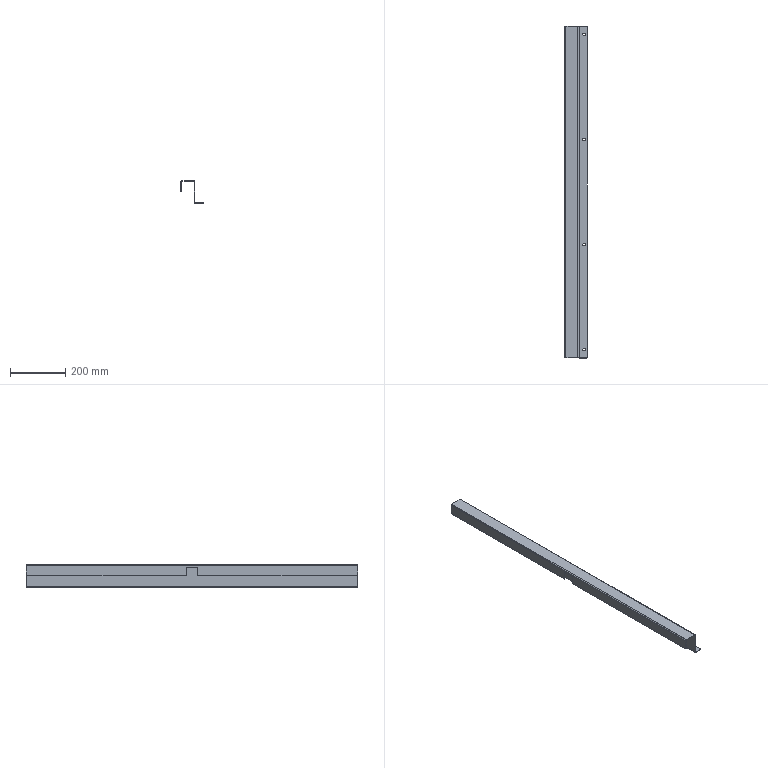Part | NX | features BREP 1 | 1 solid | 58 faces | box 80 x 1200 x 81.5 mm | volume 348715 mm3 | plane 40 | cylinder 18 | commonest cylinder face diameters 7 x15 4 x3